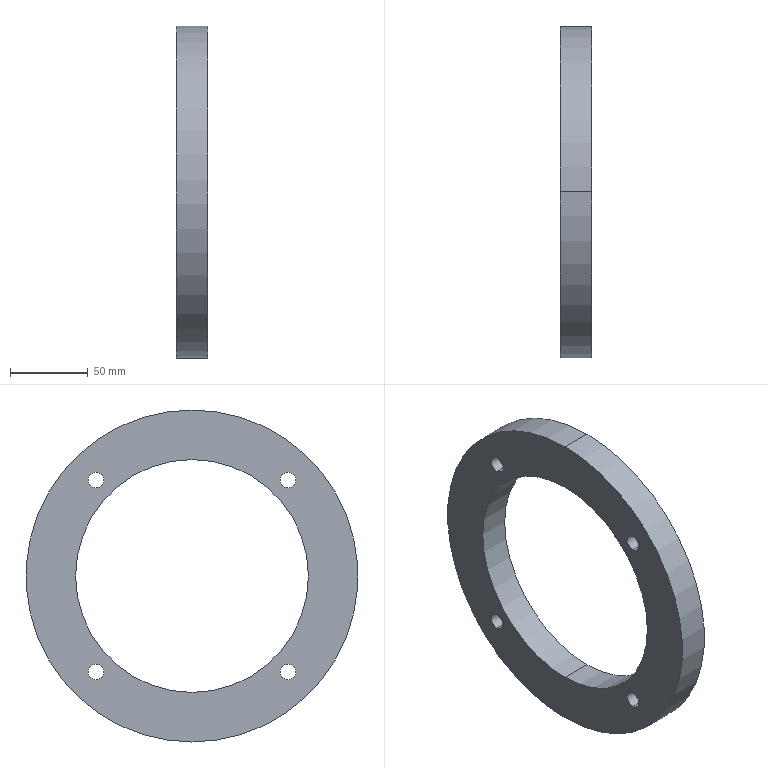Part | SolidWorks | features BaseBody 1 | 1 solid | 14 faces | box 20 x 214 x 214 mm | volume 359396 mm3 | cylinder 12 | plane 2 | commonest cylinder face diameters 10.2 x8 150 x2 214 x2
STEP:
#1=CARTESIAN_POINT('',(-10.,61.872,66.972));
#2=VERTEX_POINT('',#1);
#3=CARTESIAN_POINT('',(-10.,61.872,56.772));
#4=VERTEX_POINT('',#3);
#5=CARTESIAN_POINT('',(-10.,61.872,61.872));
#6=DIRECTION('',(1.,0.,0.));
#7=DIRECTION('',(0.,0.,-1.));
#8=AXIS2_PLACEMENT_3D('',#5,#6,#7);
#9=CIRCLE('',#8,5.1);
#10=EDGE_CURVE('',#2,#4,#9,.T.);
#11=ORIENTED_EDGE('',*,*,#10,.F.);
#12=CARTESIAN_POINT('',(10.,61.872,66.972));
#13=VERTEX_POINT('',#12);
#14=CARTESIAN_POINT('',(10.,61.872,66.972));
#15=DIRECTION('',(1.,0.,0.));
#16=VECTOR('',#15,1000.);
#17=LINE('',#14,#16);
#18=EDGE_CURVE('',#2,#13,#17,.T.);
#19=ORIENTED_EDGE('',*,*,#18,.T.);
#20=CARTESIAN_POINT('',(10.,61.872,56.772));
#21=VERTEX_POINT('',#20);
#22=CARTESIAN_POINT('',(10.,61.872,61.872));
#23=DIRECTION('',(1.,0.,0.));
#24=DIRECTION('',(0.,0.,-1.));
#25=AXIS2_PLACEMENT_3D('',#22,#23,#24);
#26=CIRCLE('',#25,5.1);
#27=EDGE_CURVE('',#13,#21,#26,.T.);
#28=ORIENTED_EDGE('',*,*,#27,.T.);
#29=CARTESIAN_POINT('',(10.,61.872,56.772));
#30=DIRECTION('',(1.,0.,0.));
#31=VECTOR('',#30,1000.);
#32=LINE('',#29,#31);
#33=EDGE_CURVE('',#4,#21,#32,.T.);
#34=ORIENTED_EDGE('',*,*,#33,.F.);
#35=EDGE_LOOP('',(#11,#19,#28,#34));
#36=FACE_OUTER_BOUND('',#35,.T.);
#37=CARTESIAN_POINT('',(10.,61.872,61.872));
#38=DIRECTION('',(1.,0.,0.));
#39=DIRECTION('',(0.,0.,-1.));
#40=AXIS2_PLACEMENT_3D('',#37,#38,#39);
#41=CYLINDRICAL_SURFACE('',#40,5.1);
#42=ADVANCED_FACE('',(#36),#41,.F.);
#43=CARTESIAN_POINT('',(-10.,61.872,-56.772));
#44=VERTEX_POINT('',#43);
#45=CARTESIAN_POINT('',(-10.,61.872,-66.972));
#46=VERTEX_POINT('',#45);
#47=CARTESIAN_POINT('',(-10.,61.872,-61.872));
#48=DIRECTION('',(1.,0.,0.));
#49=DIRECTION('',(0.,0.,-1.));
#50=AXIS2_PLACEMENT_3D('',#47,#48,#49);
#51=CIRCLE('',#50,5.1);
#52=EDGE_CURVE('',#44,#46,#51,.T.);
#53=ORIENTED_EDGE('',*,*,#52,.F.);
#54=CARTESIAN_POINT('',(10.,61.872,-56.772));
#55=VERTEX_POINT('',#54);
#56=CARTESIAN_POINT('',(10.,61.872,-56.772));
#57=DIRECTION('',(1.,0.,0.));
#58=VECTOR('',#57,1000.);
#59=LINE('',#56,#58);
#60=EDGE_CURVE('',#44,#55,#59,.T.);
#61=ORIENTED_EDGE('',*,*,#60,.T.);
#62=CARTESIAN_POINT('',(10.,61.872,-66.972));
#63=VERTEX_POINT('',#62);
#64=CARTESIAN_POINT('',(10.,61.872,-61.872));
#65=DIRECTION('',(1.,0.,0.));
#66=DIRECTION('',(0.,0.,-1.));
#67=AXIS2_PLACEMENT_3D('',#64,#65,#66);
#68=CIRCLE('',#67,5.1);
#69=EDGE_CURVE('',#55,#63,#68,.T.);
#70=ORIENTED_EDGE('',*,*,#69,.T.);
#71=CARTESIAN_POINT('',(10.,61.872,-66.972));
#72=DIRECTION('',(1.,0.,0.));
#73=VECTOR('',#72,1000.);
#74=LINE('',#71,#73);
#75=EDGE_CURVE('',#46,#63,#74,.T.);
#76=ORIENTED_EDGE('',*,*,#75,.F.);
#77=EDGE_LOOP('',(#53,#61,#70,#76));
#78=FACE_OUTER_BOUND('',#77,.T.);
#79=CARTESIAN_POINT('',(10.,61.872,-61.872));
#80=DIRECTION('',(1.,0.,0.));
#81=DIRECTION('',(0.,0.,-1.));
#82=AXIS2_PLACEMENT_3D('',#79,#80,#81);
#83=CYLINDRICAL_SURFACE('',#82,5.1);
#84=ADVANCED_FACE('',(#78),#83,.F.);
#85=CARTESIAN_POINT('',(-10.,-61.872,-56.772));
#86=VERTEX_POINT('',#85);
#87=CARTESIAN_POINT('',(-10.,-61.872,-66.972));
#88=VERTEX_POINT('',#87);
#89=CARTESIAN_POINT('',(-10.,-61.872,-61.872));
#90=DIRECTION('',(1.,0.,0.));
#91=DIRECTION('',(0.,0.,-1.));
#92=AXIS2_PLACEMENT_3D('',#89,#90,#91);
#93=CIRCLE('',#92,5.1);
#94=EDGE_CURVE('',#86,#88,#93,.T.);
#95=ORIENTED_EDGE('',*,*,#94,.F.);
#96=CARTESIAN_POINT('',(10.,-61.872,-56.772));
#97=VERTEX_POINT('',#96);
#98=CARTESIAN_POINT('',(10.,-61.872,-56.772));
#99=DIRECTION('',(1.,0.,0.));
#100=VECTOR('',#99,1000.);
#101=LINE('',#98,#100);
#102=EDGE_CURVE('',#86,#97,#101,.T.);
#103=ORIENTED_EDGE('',*,*,#102,.T.);
#104=CARTESIAN_POINT('',(10.,-61.872,-66.972));
#105=VERTEX_POINT('',#104);
#106=CARTESIAN_POINT('',(10.,-61.872,-61.872));
#107=DIRECTION('',(1.,0.,0.));
#108=DIRECTION('',(0.,0.,-1.));
#109=AXIS2_PLACEMENT_3D('',#106,#107,#108);
#110=CIRCLE('',#109,5.1);
#111=EDGE_CURVE('',#97,#105,#110,.T.);
#112=ORIENTED_EDGE('',*,*,#111,.T.);
#113=CARTESIAN_POINT('',(10.,-61.872,-66.972));
#114=DIRECTION('',(1.,0.,0.));
#115=VECTOR('',#114,1000.);
#116=LINE('',#113,#115);
#117=EDGE_CURVE('',#88,#105,#116,.T.);
#118=ORIENTED_EDGE('',*,*,#117,.F.);
#119=EDGE_LOOP('',(#95,#103,#112,#118));
#120=FACE_OUTER_BOUND('',#119,.T.);
#121=CARTESIAN_POINT('',(10.,-61.872,-61.872));
#122=DIRECTION('',(1.,0.,0.));
#123=DIRECTION('',(0.,0.,-1.));
#124=AXIS2_PLACEMENT_3D('',#121,#122,#123);
#125=CYLINDRICAL_SURFACE('',#124,5.1);
#126=ADVANCED_FACE('',(#120),#125,.F.);
#127=CARTESIAN_POINT('',(-10.,-61.872,66.972));
#128=VERTEX_POINT('',#127);
#129=CARTESIAN_POINT('',(-10.,-61.872,56.772));
#130=VERTEX_POINT('',#129);
#131=CARTESIAN_POINT('',(-10.,-61.872,61.872));
#132=DIRECTION('',(1.,0.,0.));
#133=DIRECTION('',(0.,0.,-1.));
#134=AXIS2_PLACEMENT_3D('',#131,#132,#133);
#135=CIRCLE('',#134,5.1);
#136=EDGE_CURVE('',#128,#130,#135,.T.);
#137=ORIENTED_EDGE('',*,*,#136,.F.);
#138=CARTESIAN_POINT('',(10.,-61.872,66.972));
#139=VERTEX_POINT('',#138);
#140=CARTESIAN_POINT('',(10.,-61.872,66.972));
#141=DIRECTION('',(1.,0.,0.));
#142=VECTOR('',#141,1000.);
#143=LINE('',#140,#142);
#144=EDGE_CURVE('',#128,#139,#143,.T.);
#145=ORIENTED_EDGE('',*,*,#144,.T.);
#146=CARTESIAN_POINT('',(10.,-61.872,56.772));
#147=VERTEX_POINT('',#146);
#148=CARTESIAN_POINT('',(10.,-61.872,61.872));
#149=DIRECTION('',(1.,0.,0.));
#150=DIRECTION('',(0.,0.,-1.));
#151=AXIS2_PLACEMENT_3D('',#148,#149,#150);
#152=CIRCLE('',#151,5.1);
#153=EDGE_CURVE('',#139,#147,#152,.T.);
#154=ORIENTED_EDGE('',*,*,#153,.T.);
#155=CARTESIAN_POINT('',(10.,-61.872,56.772));
#156=DIRECTION('',(1.,0.,0.));
#157=VECTOR('',#156,1000.);
#158=LINE('',#155,#157);
#159=EDGE_CURVE('',#130,#147,#158,.T.);
#160=ORIENTED_EDGE('',*,*,#159,.F.);
#161=EDGE_LOOP('',(#137,#145,#154,#160));
#162=FACE_OUTER_BOUND('',#161,.T.);
#163=CARTESIAN_POINT('',(10.,-61.872,61.872));
#164=DIRECTION('',(1.,0.,0.));
#165=DIRECTION('',(0.,0.,-1.));
#166=AXIS2_PLACEMENT_3D('',#163,#164,#165);
#167=CYLINDRICAL_SURFACE('',#166,5.1);
#168=ADVANCED_FACE('',(#162),#167,.F.);
#169=CARTESIAN_POINT('',(10.,0.,75.));
#170=VERTEX_POINT('',#169);
#171=CARTESIAN_POINT('',(10.,0.,-75.));
#172=VERTEX_POINT('',#171);
#173=CARTESIAN_POINT('',(10.,0.,0.));
#174=DIRECTION('',(1.,0.,0.));
#175=DIRECTION('',(0.,0.,-1.));
#176=AXIS2_PLACEMENT_3D('',#173,#174,#175);
#177=CIRCLE('',#176,75.);
#178=EDGE_CURVE('',#170,#172,#177,.T.);
#179=ORIENTED_EDGE('',*,*,#178,.T.);
#180=CARTESIAN_POINT('',(-10.,0.,-75.));
#181=VERTEX_POINT('',#180);
#182=CARTESIAN_POINT('',(10.,0.,-75.));
#183=DIRECTION('',(-1.,0.,0.));
#184=VECTOR('',#183,1000.);
#185=LINE('',#182,#184);
#186=EDGE_CURVE('',#172,#181,#185,.T.);
#187=ORIENTED_EDGE('',*,*,#186,.T.);
#188=CARTESIAN_POINT('',(-10.,0.,75.));
#189=VERTEX_POINT('',#188);
#190=CARTESIAN_POINT('',(-10.,0.,0.));
#191=DIRECTION('',(1.,0.,0.));
#192=DIRECTION('',(0.,0.,-1.));
#193=AXIS2_PLACEMENT_3D('',#190,#191,#192);
#194=CIRCLE('',#193,75.);
#195=EDGE_CURVE('',#189,#181,#194,.T.);
#196=ORIENTED_EDGE('',*,*,#195,.F.);
#197=CARTESIAN_POINT('',(10.,0.,75.));
#198=DIRECTION('',(-1.,0.,0.));
#199=VECTOR('',#198,1000.);
#200=LINE('',#197,#199);
#201=EDGE_CURVE('',#170,#189,#200,.T.);
#202=ORIENTED_EDGE('',*,*,#201,.F.);
#203=EDGE_LOOP('',(#179,#187,#196,#202));
#204=FACE_OUTER_BOUND('',#203,.T.);
#205=CARTESIAN_POINT('',(10.,0.,0.));
#206=DIRECTION('',(-1.,0.,0.));
#207=DIRECTION('',(0.,0.,1.));
#208=AXIS2_PLACEMENT_3D('',#205,#206,#207);
#209=CYLINDRICAL_SURFACE('',#208,75.);
#210=ADVANCED_FACE('',(#204),#209,.F.);
#211=CARTESIAN_POINT('',(10.,0.,-107.));
#212=VERTEX_POINT('',#211);
#213=CARTESIAN_POINT('',(10.,0.,107.));
#214=VERTEX_POINT('',#213);
#215=CARTESIAN_POINT('',(10.,0.,0.));
#216=DIRECTION('',(1.,0.,0.));
#217=DIRECTION('',(0.,0.,-1.));
#218=AXIS2_PLACEMENT_3D('',#215,#216,#217);
#219=CIRCLE('',#218,107.);
#220=EDGE_CURVE('',#212,#214,#219,.T.);
#221=ORIENTED_EDGE('',*,*,#220,.F.);
#222=CARTESIAN_POINT('',(-10.,0.,-107.));
#223=VERTEX_POINT('',#222);
#224=CARTESIAN_POINT('',(10.,0.,-107.));
#225=DIRECTION('',(-1.,0.,0.));
#226=VECTOR('',#225,1000.);
#227=LINE('',#224,#226);
#228=EDGE_CURVE('',#212,#223,#227,.T.);
#229=ORIENTED_EDGE('',*,*,#228,.T.);
#230=CARTESIAN_POINT('',(-10.,0.,107.));
#231=VERTEX_POINT('',#230);
#232=CARTESIAN_POINT('',(-10.,0.,0.));
#233=DIRECTION('',(1.,0.,0.));
#234=DIRECTION('',(0.,0.,-1.));
#235=AXIS2_PLACEMENT_3D('',#232,#233,#234);
#236=CIRCLE('',#235,107.);
#237=EDGE_CURVE('',#223,#231,#236,.T.);
#238=ORIENTED_EDGE('',*,*,#237,.T.);
#239=CARTESIAN_POINT('',(10.,0.,107.));
#240=DIRECTION('',(-1.,0.,0.));
#241=VECTOR('',#240,1000.);
#242=LINE('',#239,#241);
#243=EDGE_CURVE('',#214,#231,#242,.T.);
#244=ORIENTED_EDGE('',*,*,#243,.F.);
#245=EDGE_LOOP('',(#221,#229,#238,#244));
#246=FACE_OUTER_BOUND('',#245,.T.);
#247=CARTESIAN_POINT('',(10.,0.,0.));
#248=DIRECTION('',(-1.,0.,0.));
#249=DIRECTION('',(0.,0.,1.));
#250=AXIS2_PLACEMENT_3D('',#247,#248,#249);
#251=CYLINDRICAL_SURFACE('',#250,107.);
#252=ADVANCED_FACE('',(#246),#251,.T.);
#253=CARTESIAN_POINT('',(10.,61.872,61.872));
#254=DIRECTION('',(1.,0.,0.));
#255=DIRECTION('',(0.,0.,-1.));
#256=AXIS2_PLACEMENT_3D('',#253,#254,#255);
#257=CIRCLE('',#256,5.1);
#258=EDGE_CURVE('',#21,#13,#257,.T.);
#259=ORIENTED_EDGE('',*,*,#258,.F.);
#260=ORIENTED_EDGE('',*,*,#27,.F.);
#261=EDGE_LOOP('',(#259,#260));
#262=FACE_BOUND('',#261,.T.);
#263=CARTESIAN_POINT('',(10.,61.872,-61.872));
#264=DIRECTION('',(1.,0.,0.));
#265=DIRECTION('',(0.,0.,-1.));
#266=AXIS2_PLACEMENT_3D('',#263,#264,#265);
#267=CIRCLE('',#266,5.1);
#268=EDGE_CURVE('',#63,#55,#267,.T.);
#269=ORIENTED_EDGE('',*,*,#268,.F.);
#270=ORIENTED_EDGE('',*,*,#69,.F.);
#271=EDGE_LOOP('',(#269,#270));
#272=FACE_BOUND('',#271,.T.);
#273=CARTESIAN_POINT('',(10.,-61.872,-61.872));
#274=DIRECTION('',(1.,0.,0.));
#275=DIRECTION('',(0.,0.,-1.));
#276=AXIS2_PLACEMENT_3D('',#273,#274,#275);
#277=CIRCLE('',#276,5.1);
#278=EDGE_CURVE('',#105,#97,#277,.T.);
#279=ORIENTED_EDGE('',*,*,#278,.F.);
#280=ORIENTED_EDGE('',*,*,#111,.F.);
#281=EDGE_LOOP('',(#279,#280));
#282=FACE_BOUND('',#281,.T.);
#283=CARTESIAN_POINT('',(10.,-61.872,61.872));
#284=DIRECTION('',(1.,0.,0.));
#285=DIRECTION('',(0.,0.,-1.));
#286=AXIS2_PLACEMENT_3D('',#283,#284,#285);
#287=CIRCLE('',#286,5.1);
#288=EDGE_CURVE('',#147,#139,#287,.T.);
#289=ORIENTED_EDGE('',*,*,#288,.F.);
#290=ORIENTED_EDGE('',*,*,#153,.F.);
#291=EDGE_LOOP('',(#289,#290));
#292=FACE_BOUND('',#291,.T.);
#293=CARTESIAN_POINT('',(10.,0.,0.));
#294=DIRECTION('',(1.,0.,0.));
#295=DIRECTION('',(0.,0.,-1.));
#296=AXIS2_PLACEMENT_3D('',#293,#294,#295);
#297=CIRCLE('',#296,107.);
#298=EDGE_CURVE('',#214,#212,#297,.T.);
#299=ORIENTED_EDGE('',*,*,#298,.T.);
#300=ORIENTED_EDGE('',*,*,#220,.T.);
#301=EDGE_LOOP('',(#299,#300));
#302=FACE_OUTER_BOUND('',#301,.T.);
#303=ORIENTED_EDGE('',*,*,#178,.F.);
#304=CARTESIAN_POINT('',(10.,0.,0.));
#305=DIRECTION('',(1.,0.,0.));
#306=DIRECTION('',(0.,0.,-1.));
#307=AXIS2_PLACEMENT_3D('',#304,#305,#306);
#308=CIRCLE('',#307,75.);
#309=EDGE_CURVE('',#172,#170,#308,.T.);
#310=ORIENTED_EDGE('',*,*,#309,.F.);
#311=EDGE_LOOP('',(#303,#310));
#312=FACE_BOUND('',#311,.T.);
#313=CARTESIAN_POINT('',(10.,0.,0.));
#314=DIRECTION('',(1.,0.,0.));
#315=DIRECTION('',(0.,0.,-1.));
#316=AXIS2_PLACEMENT_3D('',#313,#314,#315);
#317=PLANE('',#316);
#318=ADVANCED_FACE('',(#262,#272,#282,#292,#302,#312),#317,.T.);
#319=CARTESIAN_POINT('',(-10.,61.872,61.872));
#320=DIRECTION('',(1.,0.,0.));
#321=DIRECTION('',(0.,0.,-1.));
#322=AXIS2_PLACEMENT_3D('',#319,#320,#321);
#323=CIRCLE('',#322,5.1);
#324=EDGE_CURVE('',#4,#2,#323,.T.);
#325=ORIENTED_EDGE('',*,*,#324,.T.);
#326=ORIENTED_EDGE('',*,*,#10,.T.);
#327=EDGE_LOOP('',(#325,#326));
#328=FACE_BOUND('',#327,.T.);
#329=CARTESIAN_POINT('',(-10.,61.872,-61.872));
#330=DIRECTION('',(1.,0.,0.));
#331=DIRECTION('',(0.,0.,-1.));
#332=AXIS2_PLACEMENT_3D('',#329,#330,#331);
#333=CIRCLE('',#332,5.1);
#334=EDGE_CURVE('',#46,#44,#333,.T.);
#335=ORIENTED_EDGE('',*,*,#334,.T.);
#336=ORIENTED_EDGE('',*,*,#52,.T.);
#337=EDGE_LOOP('',(#335,#336));
#338=FACE_BOUND('',#337,.T.);
#339=CARTESIAN_POINT('',(-10.,-61.872,-61.872));
#340=DIRECTION('',(1.,0.,0.));
#341=DIRECTION('',(0.,0.,-1.));
#342=AXIS2_PLACEMENT_3D('',#339,#340,#341);
#343=CIRCLE('',#342,5.1);
#344=EDGE_CURVE('',#88,#86,#343,.T.);
#345=ORIENTED_EDGE('',*,*,#344,.T.);
#346=ORIENTED_EDGE('',*,*,#94,.T.);
#347=EDGE_LOOP('',(#345,#346));
#348=FACE_BOUND('',#347,.T.);
#349=CARTESIAN_POINT('',(-10.,-61.872,61.872));
#350=DIRECTION('',(1.,0.,0.));
#351=DIRECTION('',(0.,0.,-1.));
#352=AXIS2_PLACEMENT_3D('',#349,#350,#351);
#353=CIRCLE('',#352,5.1);
#354=EDGE_CURVE('',#130,#128,#353,.T.);
#355=ORIENTED_EDGE('',*,*,#354,.T.);
#356=ORIENTED_EDGE('',*,*,#136,.T.);
#357=EDGE_LOOP('',(#355,#356));
#358=FACE_BOUND('',#357,.T.);
#359=CARTESIAN_POINT('',(-10.,0.,0.));
#360=DIRECTION('',(1.,0.,0.));
#361=DIRECTION('',(0.,0.,-1.));
#362=AXIS2_PLACEMENT_3D('',#359,#360,#361);
#363=CIRCLE('',#362,107.);
#364=EDGE_CURVE('',#231,#223,#363,.T.);
#365=ORIENTED_EDGE('',*,*,#364,.F.);
#366=ORIENTED_EDGE('',*,*,#237,.F.);
#367=EDGE_LOOP('',(#365,#366));
#368=FACE_OUTER_BOUND('',#367,.T.);
#369=ORIENTED_EDGE('',*,*,#195,.T.);
#370=CARTESIAN_POINT('',(-10.,0.,0.));
#371=DIRECTION('',(1.,0.,0.));
#372=DIRECTION('',(0.,0.,-1.));
#373=AXIS2_PLACEMENT_3D('',#370,#371,#372);
#374=CIRCLE('',#373,75.);
#375=EDGE_CURVE('',#181,#189,#374,.T.);
#376=ORIENTED_EDGE('',*,*,#375,.T.);
#377=EDGE_LOOP('',(#369,#376));
#378=FACE_BOUND('',#377,.T.);
#379=CARTESIAN_POINT('',(-10.,0.,0.));
#380=DIRECTION('',(1.,0.,0.));
#381=DIRECTION('',(0.,0.,-1.));
#382=AXIS2_PLACEMENT_3D('',#379,#380,#381);
#383=PLANE('',#382);
#384=ADVANCED_FACE('',(#328,#338,#348,#358,#368,#378),#383,.F.);
#385=ORIENTED_EDGE('',*,*,#228,.F.);
#386=ORIENTED_EDGE('',*,*,#298,.F.);
#387=ORIENTED_EDGE('',*,*,#243,.T.);
#388=ORIENTED_EDGE('',*,*,#364,.T.);
#389=EDGE_LOOP('',(#385,#386,#387,#388));
#390=FACE_OUTER_BOUND('',#389,.T.);
#391=CARTESIAN_POINT('',(10.,0.,0.));
#392=DIRECTION('',(-1.,0.,0.));
#393=DIRECTION('',(0.,0.,1.));
#394=AXIS2_PLACEMENT_3D('',#391,#392,#393);
#395=CYLINDRICAL_SURFACE('',#394,107.);
#396=ADVANCED_FACE('',(#390),#395,.T.);
#397=ORIENTED_EDGE('',*,*,#186,.F.);
#398=ORIENTED_EDGE('',*,*,#309,.T.);
#399=ORIENTED_EDGE('',*,*,#201,.T.);
#400=ORIENTED_EDGE('',*,*,#375,.F.);
#401=EDGE_LOOP('',(#397,#398,#399,#400));
#402=FACE_OUTER_BOUND('',#401,.T.);
#403=CARTESIAN_POINT('',(10.,0.,0.));
#404=DIRECTION('',(-1.,0.,0.));
#405=DIRECTION('',(0.,0.,1.));
#406=AXIS2_PLACEMENT_3D('',#403,#404,#405);
#407=CYLINDRICAL_SURFACE('',#406,75.);
#408=ADVANCED_FACE('',(#402),#407,.F.);
#409=ORIENTED_EDGE('',*,*,#144,.F.);
#410=ORIENTED_EDGE('',*,*,#354,.F.);
#411=ORIENTED_EDGE('',*,*,#159,.T.);
#412=ORIENTED_EDGE('',*,*,#288,.T.);
#413=EDGE_LOOP('',(#409,#410,#411,#412));
#414=FACE_OUTER_BOUND('',#413,.T.);
#415=CARTESIAN_POINT('',(10.,-61.872,61.872));
#416=DIRECTION('',(1.,0.,0.));
#417=DIRECTION('',(0.,0.,-1.));
#418=AXIS2_PLACEMENT_3D('',#415,#416,#417);
#419=CYLINDRICAL_SURFACE('',#418,5.1);
#420=ADVANCED_FACE('',(#414),#419,.F.);
#421=ORIENTED_EDGE('',*,*,#102,.F.);
#422=ORIENTED_EDGE('',*,*,#344,.F.);
#423=ORIENTED_EDGE('',*,*,#117,.T.);
#424=ORIENTED_EDGE('',*,*,#278,.T.);
#425=EDGE_LOOP('',(#421,#422,#423,#424));
#426=FACE_OUTER_BOUND('',#425,.T.);
#427=CARTESIAN_POINT('',(10.,-61.872,-61.872));
#428=DIRECTION('',(1.,0.,0.));
#429=DIRECTION('',(0.,0.,-1.));
#430=AXIS2_PLACEMENT_3D('',#427,#428,#429);
#431=CYLINDRICAL_SURFACE('',#430,5.1);
#432=ADVANCED_FACE('',(#426),#431,.F.);
#433=ORIENTED_EDGE('',*,*,#60,.F.);
#434=ORIENTED_EDGE('',*,*,#334,.F.);
#435=ORIENTED_EDGE('',*,*,#75,.T.);
#436=ORIENTED_EDGE('',*,*,#268,.T.);
#437=EDGE_LOOP('',(#433,#434,#435,#436));
#438=FACE_OUTER_BOUND('',#437,.T.);
#439=CARTESIAN_POINT('',(10.,61.872,-61.872));
#440=DIRECTION('',(1.,0.,0.));
#441=DIRECTION('',(0.,0.,-1.));
#442=AXIS2_PLACEMENT_3D('',#439,#440,#441);
#443=CYLINDRICAL_SURFACE('',#442,5.1);
#444=ADVANCED_FACE('',(#438),#443,.F.);
#445=ORIENTED_EDGE('',*,*,#18,.F.);
#446=ORIENTED_EDGE('',*,*,#324,.F.);
#447=ORIENTED_EDGE('',*,*,#33,.T.);
#448=ORIENTED_EDGE('',*,*,#258,.T.);
#449=EDGE_LOOP('',(#445,#446,#447,#448));
#450=FACE_OUTER_BOUND('',#449,.T.);
#451=CARTESIAN_POINT('',(10.,61.872,61.872));
#452=DIRECTION('',(1.,0.,0.));
#453=DIRECTION('',(0.,0.,-1.));
#454=AXIS2_PLACEMENT_3D('',#451,#452,#453);
#455=CYLINDRICAL_SURFACE('',#454,5.1);
#456=ADVANCED_FACE('',(#450),#455,.F.);
#457=CLOSED_SHELL('',(#42,#84,#126,#168,#210,#252,#318,#384,#396,#408,#420,#432,#444,#456));
#458=MANIFOLD_SOLID_BREP('',#457);
#459=CARTESIAN_POINT('',(0.,0.,0.));
#460=DIRECTION('',(0.,0.,1.));
#461=DIRECTION('',(1.,0.,0.));
#462=AXIS2_PLACEMENT_3D('',#459,#460,#461);
#463=(LENGTH_UNIT()NAMED_UNIT(*)SI_UNIT(.MILLI.,.METRE.));
#464=UNCERTAINTY_MEASURE_WITH_UNIT(LENGTH_MEASURE(0.00001),#463,'','');
#465=(NAMED_UNIT(*)PLANE_ANGLE_UNIT()SI_UNIT($,.RADIAN.));
#466=(NAMED_UNIT(*)SI_UNIT($,.STERADIAN.)SOLID_ANGLE_UNIT());
#467=(GEOMETRIC_REPRESENTATION_CONTEXT(3)GLOBAL_UNCERTAINTY_ASSIGNED_CONTEXT((#464))GLOBAL_UNIT_ASSIGNED_CONTEXT((#463,#465,#466))REPRESENTATION_CONTEXT('',''));
#468=ADVANCED_BREP_SHAPE_REPRESENTATION('',(#458,#462),#467);